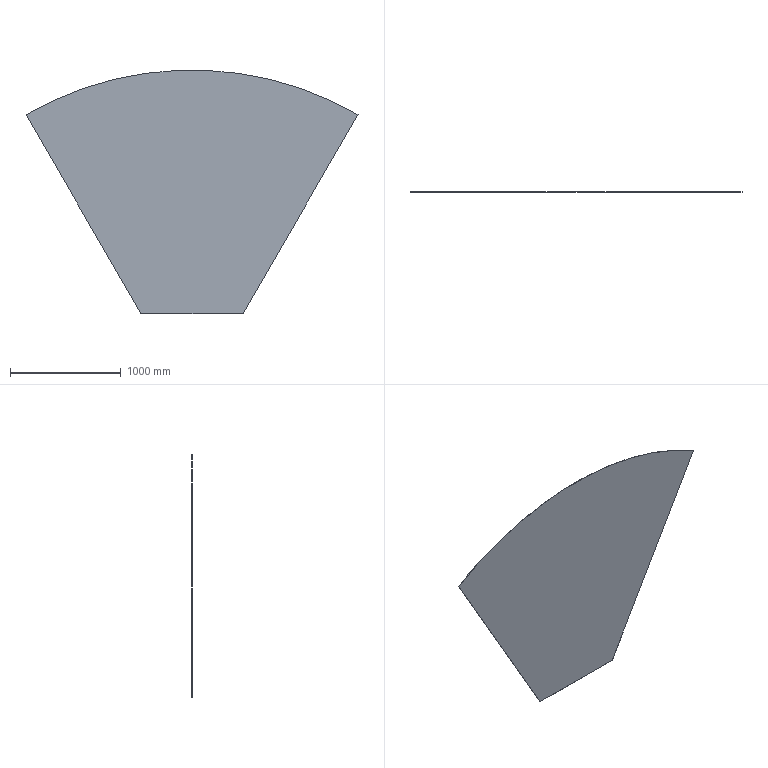Part | SolidWorks | features Extrusion 1 | 1 solid | 6 faces | box 3000 x 3 x 2200 mm | volume 13028079 mm3 | plane 5 | cylinder 1 | commonest cylinder face diameters 6000 x1
STEP:
#1=CARTESIAN_POINT('',(1500.,0.,1797.869));
#2=VERTEX_POINT('',#1);
#3=CARTESIAN_POINT('',(462.,0.,0.));
#4=VERTEX_POINT('',#3);
#5=CARTESIAN_POINT('',(462.,0.,0.));
#6=DIRECTION('',(-0.5,0.,-0.866));
#7=VECTOR('',#6,1000.);
#8=LINE('',#5,#7);
#9=EDGE_CURVE('',#2,#4,#8,.T.);
#10=ORIENTED_EDGE('',*,*,#9,.T.);
#11=CARTESIAN_POINT('',(462.,3.,0.));
#12=VERTEX_POINT('',#11);
#13=CARTESIAN_POINT('',(462.,3.,0.));
#14=DIRECTION('',(0.,-1.,0.));
#15=VECTOR('',#14,1000.);
#16=LINE('',#13,#15);
#17=EDGE_CURVE('',#12,#4,#16,.T.);
#18=ORIENTED_EDGE('',*,*,#17,.F.);
#19=CARTESIAN_POINT('',(1500.,3.,1797.869));
#20=VERTEX_POINT('',#19);
#21=CARTESIAN_POINT('',(462.,3.,0.));
#22=DIRECTION('',(-0.5,0.,-0.866));
#23=VECTOR('',#22,1000.);
#24=LINE('',#21,#23);
#25=EDGE_CURVE('',#20,#12,#24,.T.);
#26=ORIENTED_EDGE('',*,*,#25,.F.);
#27=CARTESIAN_POINT('',(1500.,3.,1797.869));
#28=DIRECTION('',(0.,-1.,0.));
#29=VECTOR('',#28,1000.);
#30=LINE('',#27,#29);
#31=EDGE_CURVE('',#20,#2,#30,.T.);
#32=ORIENTED_EDGE('',*,*,#31,.T.);
#33=EDGE_LOOP('',(#10,#18,#26,#32));
#34=FACE_OUTER_BOUND('',#33,.T.);
#35=CARTESIAN_POINT('',(462.,3.,0.));
#36=DIRECTION('',(-0.866,0.,0.5));
#37=DIRECTION('',(0.5,0.,0.866));
#38=AXIS2_PLACEMENT_3D('',#35,#36,#37);
#39=PLANE('',#38);
#40=ADVANCED_FACE('',(#34),#39,.F.);
#41=CARTESIAN_POINT('',(-462.,0.,0.));
#42=VERTEX_POINT('',#41);
#43=CARTESIAN_POINT('',(-462.,0.,0.));
#44=DIRECTION('',(-1.,0.,0.));
#45=VECTOR('',#44,1000.);
#46=LINE('',#43,#45);
#47=EDGE_CURVE('',#4,#42,#46,.T.);
#48=ORIENTED_EDGE('',*,*,#47,.T.);
#49=CARTESIAN_POINT('',(-462.,3.,0.));
#50=VERTEX_POINT('',#49);
#51=CARTESIAN_POINT('',(-462.,3.,0.));
#52=DIRECTION('',(0.,-1.,0.));
#53=VECTOR('',#52,1000.);
#54=LINE('',#51,#53);
#55=EDGE_CURVE('',#50,#42,#54,.T.);
#56=ORIENTED_EDGE('',*,*,#55,.F.);
#57=CARTESIAN_POINT('',(-462.,3.,0.));
#58=DIRECTION('',(-1.,0.,0.));
#59=VECTOR('',#58,1000.);
#60=LINE('',#57,#59);
#61=EDGE_CURVE('',#12,#50,#60,.T.);
#62=ORIENTED_EDGE('',*,*,#61,.F.);
#63=ORIENTED_EDGE('',*,*,#17,.T.);
#64=EDGE_LOOP('',(#48,#56,#62,#63));
#65=FACE_OUTER_BOUND('',#64,.T.);
#66=CARTESIAN_POINT('',(-462.,3.,0.));
#67=DIRECTION('',(0.,0.,1.));
#68=DIRECTION('',(1.,0.,0.));
#69=AXIS2_PLACEMENT_3D('',#66,#67,#68);
#70=PLANE('',#69);
#71=ADVANCED_FACE('',(#65),#70,.F.);
#72=CARTESIAN_POINT('',(-1500.,0.,1797.869));
#73=VERTEX_POINT('',#72);
#74=CARTESIAN_POINT('',(-462.,0.,0.));
#75=DIRECTION('',(-0.5,0.,0.866));
#76=VECTOR('',#75,1000.);
#77=LINE('',#74,#76);
#78=EDGE_CURVE('',#42,#73,#77,.T.);
#79=ORIENTED_EDGE('',*,*,#78,.T.);
#80=CARTESIAN_POINT('',(-1500.,3.,1797.869));
#81=VERTEX_POINT('',#80);
#82=CARTESIAN_POINT('',(-1500.,3.,1797.869));
#83=DIRECTION('',(0.,-1.,0.));
#84=VECTOR('',#83,1000.);
#85=LINE('',#82,#84);
#86=EDGE_CURVE('',#81,#73,#85,.T.);
#87=ORIENTED_EDGE('',*,*,#86,.F.);
#88=CARTESIAN_POINT('',(-462.,3.,0.));
#89=DIRECTION('',(-0.5,0.,0.866));
#90=VECTOR('',#89,1000.);
#91=LINE('',#88,#90);
#92=EDGE_CURVE('',#50,#81,#91,.T.);
#93=ORIENTED_EDGE('',*,*,#92,.F.);
#94=ORIENTED_EDGE('',*,*,#55,.T.);
#95=EDGE_LOOP('',(#79,#87,#93,#94));
#96=FACE_OUTER_BOUND('',#95,.T.);
#97=CARTESIAN_POINT('',(-462.,3.,0.));
#98=DIRECTION('',(0.866,0.,0.5));
#99=DIRECTION('',(0.5,0.,-0.866));
#100=AXIS2_PLACEMENT_3D('',#97,#98,#99);
#101=PLANE('',#100);
#102=ADVANCED_FACE('',(#96),#101,.F.);
#103=CARTESIAN_POINT('',(0.,0.,-800.207));
#104=DIRECTION('',(0.,1.,0.));
#105=DIRECTION('',(0.,0.,1.));
#106=AXIS2_PLACEMENT_3D('',#103,#104,#105);
#107=CIRCLE('',#106,3000.);
#108=EDGE_CURVE('',#73,#2,#107,.T.);
#109=ORIENTED_EDGE('',*,*,#108,.T.);
#110=ORIENTED_EDGE('',*,*,#31,.F.);
#111=CARTESIAN_POINT('',(0.,3.,-800.207));
#112=DIRECTION('',(0.,1.,0.));
#113=DIRECTION('',(0.,0.,1.));
#114=AXIS2_PLACEMENT_3D('',#111,#112,#113);
#115=CIRCLE('',#114,3000.);
#116=EDGE_CURVE('',#81,#20,#115,.T.);
#117=ORIENTED_EDGE('',*,*,#116,.F.);
#118=ORIENTED_EDGE('',*,*,#86,.T.);
#119=EDGE_LOOP('',(#109,#110,#117,#118));
#120=FACE_OUTER_BOUND('',#119,.T.);
#121=CARTESIAN_POINT('',(0.,3.,-800.207));
#122=DIRECTION('',(0.,-1.,0.));
#123=DIRECTION('',(0.,0.,-1.));
#124=AXIS2_PLACEMENT_3D('',#121,#122,#123);
#125=CYLINDRICAL_SURFACE('',#124,3000.);
#126=ADVANCED_FACE('',(#120),#125,.T.);
#127=ORIENTED_EDGE('',*,*,#25,.T.);
#128=ORIENTED_EDGE('',*,*,#61,.T.);
#129=ORIENTED_EDGE('',*,*,#92,.T.);
#130=ORIENTED_EDGE('',*,*,#116,.T.);
#131=EDGE_LOOP('',(#127,#128,#129,#130));
#132=FACE_OUTER_BOUND('',#131,.T.);
#133=CARTESIAN_POINT('',(0.,3.,-800.207));
#134=DIRECTION('',(0.,1.,0.));
#135=DIRECTION('',(0.,0.,1.));
#136=AXIS2_PLACEMENT_3D('',#133,#134,#135);
#137=PLANE('',#136);
#138=ADVANCED_FACE('',(#132),#137,.T.);
#139=ORIENTED_EDGE('',*,*,#9,.F.);
#140=ORIENTED_EDGE('',*,*,#108,.F.);
#141=ORIENTED_EDGE('',*,*,#78,.F.);
#142=ORIENTED_EDGE('',*,*,#47,.F.);
#143=EDGE_LOOP('',(#139,#140,#141,#142));
#144=FACE_OUTER_BOUND('',#143,.T.);
#145=CARTESIAN_POINT('',(0.,0.,-800.207));
#146=DIRECTION('',(0.,1.,0.));
#147=DIRECTION('',(0.,0.,1.));
#148=AXIS2_PLACEMENT_3D('',#145,#146,#147);
#149=PLANE('',#148);
#150=ADVANCED_FACE('',(#144),#149,.F.);
#151=CLOSED_SHELL('',(#40,#71,#102,#126,#138,#150));
#152=MANIFOLD_SOLID_BREP('',#151);
#153=CARTESIAN_POINT('',(0.,0.,0.));
#154=DIRECTION('',(0.,0.,1.));
#155=DIRECTION('',(1.,0.,0.));
#156=AXIS2_PLACEMENT_3D('',#153,#154,#155);
#157=(LENGTH_UNIT()NAMED_UNIT(*)SI_UNIT(.MILLI.,.METRE.));
#158=UNCERTAINTY_MEASURE_WITH_UNIT(LENGTH_MEASURE(0.00001),#157,'','');
#159=(NAMED_UNIT(*)PLANE_ANGLE_UNIT()SI_UNIT($,.RADIAN.));
#160=(NAMED_UNIT(*)SI_UNIT($,.STERADIAN.)SOLID_ANGLE_UNIT());
#161=(GEOMETRIC_REPRESENTATION_CONTEXT(3)GLOBAL_UNCERTAINTY_ASSIGNED_CONTEXT((#158))GLOBAL_UNIT_ASSIGNED_CONTEXT((#157,#159,#160))REPRESENTATION_CONTEXT('',''));
#162=ADVANCED_BREP_SHAPE_REPRESENTATION('',(#152,#156),#161);